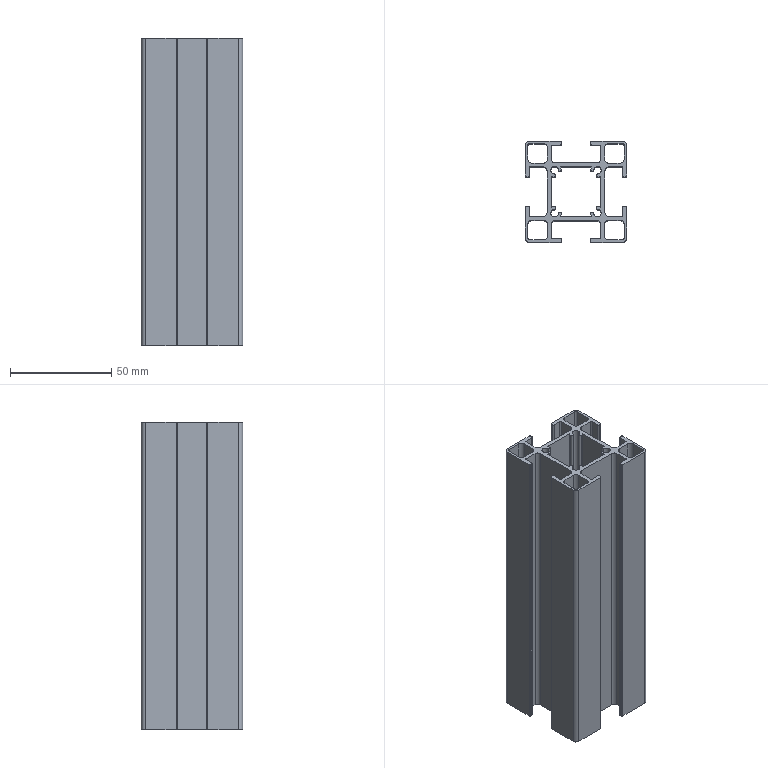Part | STEP file | 46A-00006CC11-152mm | 1 solid | 142 faces | box 50 x 50 x 152 mm | volume 89299 mm3 | cylinder 84 | plane 58 | commonest cylinder face diameters 1 x24 4 x24 1.5 x16 3.7 x8 6.7 x8 2 x4